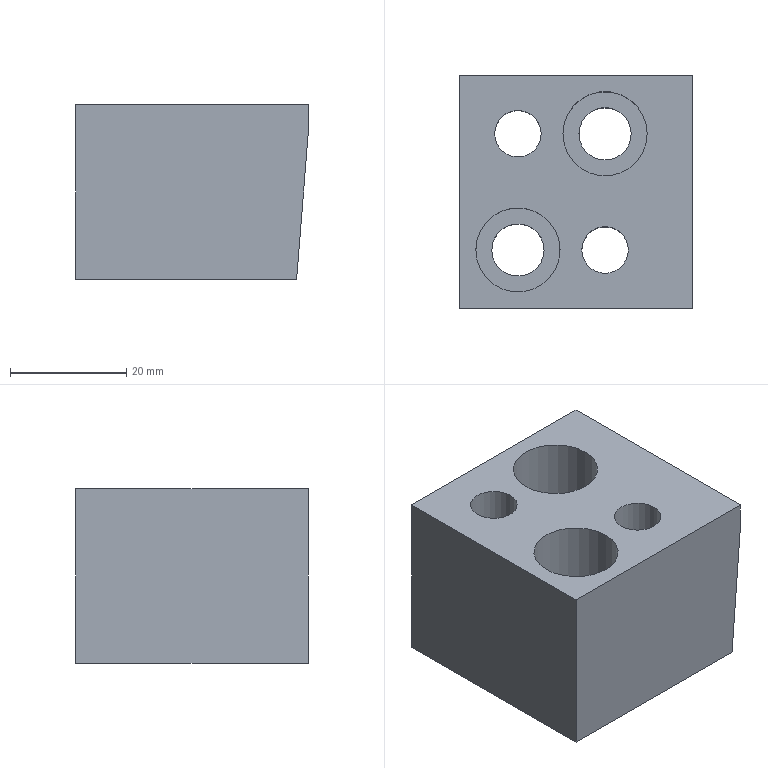Part | NX | features 23 2 | 1 solid | 15 faces | box 40 x 40 x 30 mm | volume 37933 mm3 | plane 9 | cylinder 6 | commonest cylinder face diameters 8.001 x2 9 x2 14.5 x2
STEP:
#1=CARTESIAN_POINT('',(3683.056,10.,-3.5));
#2=VERTEX_POINT('',#1);
#3=CARTESIAN_POINT('',(3675.806,10.,-3.5));
#4=DIRECTION('',(0.,0.,-1.));
#5=DIRECTION('',(1.,0.,0.));
#6=AXIS2_PLACEMENT_3D('',#3,#4,#5);
#7=CIRCLE('',#6,7.25);
#8=EDGE_CURVE('',#2,#2,#7,.T.);
#9=ORIENTED_EDGE('',*,*,#8,.T.);
#10=EDGE_LOOP('',(#9));
#11=FACE_BOUND('',#10,.T.);
#12=CARTESIAN_POINT('',(3690.806,-20.,-3.5));
#13=VERTEX_POINT('',#12);
#14=CARTESIAN_POINT('',(3650.806,-20.,-3.5));
#15=VERTEX_POINT('',#14);
#16=CARTESIAN_POINT('',(3675.806,-20.,-3.5));
#17=DIRECTION('',(-1.,0.,0.));
#18=VECTOR('',#17,1000.);
#19=LINE('',#16,#18);
#20=EDGE_CURVE('',#13,#15,#19,.T.);
#21=ORIENTED_EDGE('',*,*,#20,.F.);
#22=CARTESIAN_POINT('',(3690.806,20.,-3.5));
#23=VERTEX_POINT('',#22);
#24=CARTESIAN_POINT('',(3690.806,0.,-3.5));
#25=DIRECTION('',(0.,-1.,0.));
#26=VECTOR('',#25,1000.);
#27=LINE('',#24,#26);
#28=EDGE_CURVE('',#23,#13,#27,.T.);
#29=ORIENTED_EDGE('',*,*,#28,.F.);
#30=CARTESIAN_POINT('',(3650.806,20.,-3.5));
#31=VERTEX_POINT('',#30);
#32=CARTESIAN_POINT('',(3675.806,20.,-3.5));
#33=DIRECTION('',(1.,0.,0.));
#34=VECTOR('',#33,1000.);
#35=LINE('',#32,#34);
#36=EDGE_CURVE('',#31,#23,#35,.T.);
#37=ORIENTED_EDGE('',*,*,#36,.F.);
#38=CARTESIAN_POINT('',(3650.806,0.,-3.5));
#39=DIRECTION('',(0.,1.,0.));
#40=VECTOR('',#39,1000.);
#41=LINE('',#38,#40);
#42=EDGE_CURVE('',#15,#31,#41,.T.);
#43=ORIENTED_EDGE('',*,*,#42,.F.);
#44=EDGE_LOOP('',(#21,#29,#37,#43));
#45=FACE_BOUND('',#44,.T.);
#46=CARTESIAN_POINT('',(3664.807,10.,-3.5));
#47=VERTEX_POINT('',#46);
#48=CARTESIAN_POINT('',(3660.806,10.,-3.5));
#49=DIRECTION('',(0.,0.,1.));
#50=DIRECTION('',(1.,0.,0.));
#51=AXIS2_PLACEMENT_3D('',#48,#49,#50);
#52=CIRCLE('',#51,4.);
#53=EDGE_CURVE('',#47,#47,#52,.T.);
#54=ORIENTED_EDGE('',*,*,#53,.F.);
#55=EDGE_LOOP('',(#54));
#56=FACE_BOUND('',#55,.T.);
#57=CARTESIAN_POINT('',(3679.807,-10.,-3.5));
#58=VERTEX_POINT('',#57);
#59=CARTESIAN_POINT('',(3675.806,-10.,-3.5));
#60=DIRECTION('',(0.,0.,1.));
#61=DIRECTION('',(1.,0.,0.));
#62=AXIS2_PLACEMENT_3D('',#59,#60,#61);
#63=CIRCLE('',#62,4.);
#64=EDGE_CURVE('',#58,#58,#63,.T.);
#65=ORIENTED_EDGE('',*,*,#64,.F.);
#66=EDGE_LOOP('',(#65));
#67=FACE_BOUND('',#66,.T.);
#68=CARTESIAN_POINT('',(3668.056,-10.,-3.5));
#69=VERTEX_POINT('',#68);
#70=CARTESIAN_POINT('',(3660.806,-10.,-3.5));
#71=DIRECTION('',(0.,0.,-1.));
#72=DIRECTION('',(1.,0.,0.));
#73=AXIS2_PLACEMENT_3D('',#70,#71,#72);
#74=CIRCLE('',#73,7.25);
#75=EDGE_CURVE('',#69,#69,#74,.T.);
#76=ORIENTED_EDGE('',*,*,#75,.T.);
#77=EDGE_LOOP('',(#76));
#78=FACE_BOUND('',#77,.T.);
#79=CARTESIAN_POINT('',(3675.806,0.,-3.5));
#80=DIRECTION('',(0.,0.,1.));
#81=DIRECTION('',(-1.,0.,0.));
#82=AXIS2_PLACEMENT_3D('',#79,#80,#81);
#83=PLANE('',#82);
#84=ADVANCED_FACE('',(#11,#45,#56,#67,#78),#83,.T.);
#85=CARTESIAN_POINT('',(3650.806,-20.,-33.5));
#86=VERTEX_POINT('',#85);
#87=CARTESIAN_POINT('',(3688.806,-20.,-33.5));
#88=VERTEX_POINT('',#87);
#89=CARTESIAN_POINT('',(3675.806,-20.,-33.5));
#90=DIRECTION('',(1.,0.,0.));
#91=VECTOR('',#90,1000.);
#92=LINE('',#89,#91);
#93=EDGE_CURVE('',#86,#88,#92,.T.);
#94=ORIENTED_EDGE('',*,*,#93,.T.);
#95=CARTESIAN_POINT('',(3690.806,-20.,-8.5));
#96=VERTEX_POINT('',#95);
#97=CARTESIAN_POINT('',(3688.724,-20.,-34.533));
#98=DIRECTION('',(0.07975,0.,0.9968));
#99=VECTOR('',#98,1000.);
#100=LINE('',#97,#99);
#101=EDGE_CURVE('',#88,#96,#100,.T.);
#102=ORIENTED_EDGE('',*,*,#101,.T.);
#103=CARTESIAN_POINT('',(3690.806,-20.,-33.5));
#104=DIRECTION('',(0.,0.,1.));
#105=VECTOR('',#104,1000.);
#106=LINE('',#103,#105);
#107=EDGE_CURVE('',#96,#13,#106,.T.);
#108=ORIENTED_EDGE('',*,*,#107,.T.);
#109=ORIENTED_EDGE('',*,*,#20,.T.);
#110=CARTESIAN_POINT('',(3650.806,-20.,-33.5));
#111=DIRECTION('',(0.,0.,1.));
#112=VECTOR('',#111,1000.);
#113=LINE('',#110,#112);
#114=EDGE_CURVE('',#86,#15,#113,.T.);
#115=ORIENTED_EDGE('',*,*,#114,.F.);
#116=EDGE_LOOP('',(#94,#102,#108,#109,#115));
#117=FACE_BOUND('',#116,.T.);
#118=CARTESIAN_POINT('',(3675.806,-20.,-33.5));
#119=DIRECTION('',(0.,-1.,0.));
#120=DIRECTION('',(0.,0.,1.));
#121=AXIS2_PLACEMENT_3D('',#118,#119,#120);
#122=PLANE('',#121);
#123=ADVANCED_FACE('',(#117),#122,.T.);
#124=ORIENTED_EDGE('',*,*,#114,.T.);
#125=ORIENTED_EDGE('',*,*,#42,.T.);
#126=CARTESIAN_POINT('',(3650.806,20.,-33.5));
#127=VERTEX_POINT('',#126);
#128=CARTESIAN_POINT('',(3650.806,20.,-33.5));
#129=DIRECTION('',(0.,0.,1.));
#130=VECTOR('',#129,1000.);
#131=LINE('',#128,#130);
#132=EDGE_CURVE('',#127,#31,#131,.T.);
#133=ORIENTED_EDGE('',*,*,#132,.F.);
#134=CARTESIAN_POINT('',(3650.806,0.,-33.5));
#135=DIRECTION('',(0.,-1.,0.));
#136=VECTOR('',#135,1000.);
#137=LINE('',#134,#136);
#138=EDGE_CURVE('',#127,#86,#137,.T.);
#139=ORIENTED_EDGE('',*,*,#138,.T.);
#140=EDGE_LOOP('',(#124,#125,#133,#139));
#141=FACE_BOUND('',#140,.T.);
#142=CARTESIAN_POINT('',(3650.806,0.,-33.5));
#143=DIRECTION('',(-1.,0.,0.));
#144=DIRECTION('',(0.,0.,-1.));
#145=AXIS2_PLACEMENT_3D('',#142,#143,#144);
#146=PLANE('',#145);
#147=ADVANCED_FACE('',(#141),#146,.T.);
#148=CARTESIAN_POINT('',(3690.806,20.,-8.5));
#149=VERTEX_POINT('',#148);
#150=CARTESIAN_POINT('',(3690.806,20.,-33.5));
#151=DIRECTION('',(0.,0.,1.));
#152=VECTOR('',#151,1000.);
#153=LINE('',#150,#152);
#154=EDGE_CURVE('',#149,#23,#153,.T.);
#155=ORIENTED_EDGE('',*,*,#154,.F.);
#156=CARTESIAN_POINT('',(3688.806,20.,-33.5));
#157=VERTEX_POINT('',#156);
#158=CARTESIAN_POINT('',(3688.724,20.,-34.533));
#159=DIRECTION('',(-0.07975,0.,-0.9968));
#160=VECTOR('',#159,1000.);
#161=LINE('',#158,#160);
#162=EDGE_CURVE('',#149,#157,#161,.T.);
#163=ORIENTED_EDGE('',*,*,#162,.T.);
#164=CARTESIAN_POINT('',(3675.806,20.,-33.5));
#165=DIRECTION('',(-1.,0.,0.));
#166=VECTOR('',#165,1000.);
#167=LINE('',#164,#166);
#168=EDGE_CURVE('',#157,#127,#167,.T.);
#169=ORIENTED_EDGE('',*,*,#168,.T.);
#170=ORIENTED_EDGE('',*,*,#132,.T.);
#171=ORIENTED_EDGE('',*,*,#36,.T.);
#172=EDGE_LOOP('',(#155,#163,#169,#170,#171));
#173=FACE_BOUND('',#172,.T.);
#174=CARTESIAN_POINT('',(3675.806,20.,-33.5));
#175=DIRECTION('',(0.,1.,0.));
#176=DIRECTION('',(0.,0.,-1.));
#177=AXIS2_PLACEMENT_3D('',#174,#175,#176);
#178=PLANE('',#177);
#179=ADVANCED_FACE('',(#173),#178,.T.);
#180=CARTESIAN_POINT('',(3656.306,-10.,-33.5));
#181=VERTEX_POINT('',#180);
#182=CARTESIAN_POINT('',(3660.806,-10.,-33.5));
#183=DIRECTION('',(0.,0.,-1.));
#184=DIRECTION('',(-1.,0.,0.));
#185=AXIS2_PLACEMENT_3D('',#182,#183,#184);
#186=CIRCLE('',#185,4.5);
#187=EDGE_CURVE('',#181,#181,#186,.T.);
#188=ORIENTED_EDGE('',*,*,#187,.F.);
#189=EDGE_LOOP('',(#188));
#190=FACE_BOUND('',#189,.T.);
#191=CARTESIAN_POINT('',(3671.806,-10.,-33.5));
#192=VERTEX_POINT('',#191);
#193=CARTESIAN_POINT('',(3675.806,-10.,-33.5));
#194=DIRECTION('',(0.,0.,-1.));
#195=DIRECTION('',(-1.,0.,0.));
#196=AXIS2_PLACEMENT_3D('',#193,#194,#195);
#197=CIRCLE('',#196,4.);
#198=EDGE_CURVE('',#192,#192,#197,.T.);
#199=ORIENTED_EDGE('',*,*,#198,.F.);
#200=EDGE_LOOP('',(#199));
#201=FACE_BOUND('',#200,.T.);
#202=CARTESIAN_POINT('',(3656.806,10.,-33.5));
#203=VERTEX_POINT('',#202);
#204=CARTESIAN_POINT('',(3660.806,10.,-33.5));
#205=DIRECTION('',(0.,0.,-1.));
#206=DIRECTION('',(-1.,0.,0.));
#207=AXIS2_PLACEMENT_3D('',#204,#205,#206);
#208=CIRCLE('',#207,4.);
#209=EDGE_CURVE('',#203,#203,#208,.T.);
#210=ORIENTED_EDGE('',*,*,#209,.F.);
#211=EDGE_LOOP('',(#210));
#212=FACE_BOUND('',#211,.T.);
#213=CARTESIAN_POINT('',(3671.306,10.,-33.5));
#214=VERTEX_POINT('',#213);
#215=CARTESIAN_POINT('',(3675.806,10.,-33.5));
#216=DIRECTION('',(0.,0.,-1.));
#217=DIRECTION('',(-1.,0.,0.));
#218=AXIS2_PLACEMENT_3D('',#215,#216,#217);
#219=CIRCLE('',#218,4.5);
#220=EDGE_CURVE('',#214,#214,#219,.T.);
#221=ORIENTED_EDGE('',*,*,#220,.F.);
#222=EDGE_LOOP('',(#221));
#223=FACE_BOUND('',#222,.T.);
#224=ORIENTED_EDGE('',*,*,#168,.F.);
#225=CARTESIAN_POINT('',(3688.806,0.,-33.5));
#226=DIRECTION('',(0.,-1.,0.));
#227=VECTOR('',#226,1000.);
#228=LINE('',#225,#227);
#229=EDGE_CURVE('',#157,#88,#228,.T.);
#230=ORIENTED_EDGE('',*,*,#229,.T.);
#231=ORIENTED_EDGE('',*,*,#93,.F.);
#232=ORIENTED_EDGE('',*,*,#138,.F.);
#233=EDGE_LOOP('',(#224,#230,#231,#232));
#234=FACE_BOUND('',#233,.T.);
#235=CARTESIAN_POINT('',(3675.806,0.,-33.5));
#236=DIRECTION('',(0.,0.,-1.));
#237=DIRECTION('',(1.,0.,0.));
#238=AXIS2_PLACEMENT_3D('',#235,#236,#237);
#239=PLANE('',#238);
#240=ADVANCED_FACE('',(#190,#201,#212,#223,#234),#239,.T.);
#241=ORIENTED_EDGE('',*,*,#107,.F.);
#242=CARTESIAN_POINT('',(3690.806,0.,-8.5));
#243=DIRECTION('',(0.,1.,0.));
#244=VECTOR('',#243,1000.);
#245=LINE('',#242,#244);
#246=EDGE_CURVE('',#96,#149,#245,.T.);
#247=ORIENTED_EDGE('',*,*,#246,.T.);
#248=ORIENTED_EDGE('',*,*,#154,.T.);
#249=ORIENTED_EDGE('',*,*,#28,.T.);
#250=EDGE_LOOP('',(#241,#247,#248,#249));
#251=FACE_BOUND('',#250,.T.);
#252=CARTESIAN_POINT('',(3690.806,0.,-33.5));
#253=DIRECTION('',(1.,0.,0.));
#254=DIRECTION('',(0.,0.,1.));
#255=AXIS2_PLACEMENT_3D('',#252,#253,#254);
#256=PLANE('',#255);
#257=ADVANCED_FACE('',(#251),#256,.T.);
#258=ORIENTED_EDGE('',*,*,#220,.T.);
#259=EDGE_LOOP('',(#258));
#260=FACE_BOUND('',#259,.T.);
#261=CARTESIAN_POINT('',(3671.306,10.,-14.5));
#262=VERTEX_POINT('',#261);
#263=CARTESIAN_POINT('',(3675.806,10.,-14.5));
#264=DIRECTION('',(0.,0.,-1.));
#265=DIRECTION('',(-1.,0.,0.));
#266=AXIS2_PLACEMENT_3D('',#263,#264,#265);
#267=CIRCLE('',#266,4.5);
#268=EDGE_CURVE('',#262,#262,#267,.T.);
#269=ORIENTED_EDGE('',*,*,#268,.F.);
#270=EDGE_LOOP('',(#269));
#271=FACE_BOUND('',#270,.T.);
#272=CARTESIAN_POINT('',(3675.806,10.,-1.5));
#273=DIRECTION('',(0.,0.,-1.));
#274=DIRECTION('',(-1.,0.,0.));
#275=AXIS2_PLACEMENT_3D('',#272,#273,#274);
#276=CYLINDRICAL_SURFACE('',#275,4.5);
#277=ADVANCED_FACE('',(#260,#271),#276,.F.);
#278=ORIENTED_EDGE('',*,*,#268,.T.);
#279=EDGE_LOOP('',(#278));
#280=FACE_BOUND('',#279,.T.);
#281=CARTESIAN_POINT('',(3683.056,10.,-14.5));
#282=VERTEX_POINT('',#281);
#283=CARTESIAN_POINT('',(3675.806,10.,-14.5));
#284=DIRECTION('',(0.,0.,-1.));
#285=DIRECTION('',(1.,0.,0.));
#286=AXIS2_PLACEMENT_3D('',#283,#284,#285);
#287=CIRCLE('',#286,7.25);
#288=EDGE_CURVE('',#282,#282,#287,.T.);
#289=ORIENTED_EDGE('',*,*,#288,.F.);
#290=EDGE_LOOP('',(#289));
#291=FACE_BOUND('',#290,.T.);
#292=CARTESIAN_POINT('',(3675.806,10.,-14.5));
#293=DIRECTION('',(0.,0.,-1.));
#294=DIRECTION('',(1.,0.,0.));
#295=AXIS2_PLACEMENT_3D('',#292,#293,#294);
#296=PLANE('',#295);
#297=ADVANCED_FACE('',(#280,#291),#296,.F.);
#298=ORIENTED_EDGE('',*,*,#288,.T.);
#299=EDGE_LOOP('',(#298));
#300=FACE_BOUND('',#299,.T.);
#301=ORIENTED_EDGE('',*,*,#8,.F.);
#302=EDGE_LOOP('',(#301));
#303=FACE_BOUND('',#302,.T.);
#304=CARTESIAN_POINT('',(3675.806,10.,-3.5));
#305=DIRECTION('',(0.,0.,-1.));
#306=DIRECTION('',(-1.,0.,0.));
#307=AXIS2_PLACEMENT_3D('',#304,#305,#306);
#308=CYLINDRICAL_SURFACE('',#307,7.25);
#309=ADVANCED_FACE('',(#300,#303),#308,.F.);
#310=ORIENTED_EDGE('',*,*,#53,.T.);
#311=EDGE_LOOP('',(#310));
#312=FACE_BOUND('',#311,.T.);
#313=ORIENTED_EDGE('',*,*,#209,.T.);
#314=EDGE_LOOP('',(#313));
#315=FACE_BOUND('',#314,.T.);
#316=CARTESIAN_POINT('',(3660.806,10.,-1.5));
#317=DIRECTION('',(0.,0.,-1.));
#318=DIRECTION('',(-1.,0.,0.));
#319=AXIS2_PLACEMENT_3D('',#316,#317,#318);
#320=CYLINDRICAL_SURFACE('',#319,4.);
#321=ADVANCED_FACE('',(#312,#315),#320,.F.);
#322=ORIENTED_EDGE('',*,*,#64,.T.);
#323=EDGE_LOOP('',(#322));
#324=FACE_BOUND('',#323,.T.);
#325=ORIENTED_EDGE('',*,*,#198,.T.);
#326=EDGE_LOOP('',(#325));
#327=FACE_BOUND('',#326,.T.);
#328=CARTESIAN_POINT('',(3675.806,-10.,-1.5));
#329=DIRECTION('',(0.,0.,-1.));
#330=DIRECTION('',(-1.,0.,0.));
#331=AXIS2_PLACEMENT_3D('',#328,#329,#330);
#332=CYLINDRICAL_SURFACE('',#331,4.);
#333=ADVANCED_FACE('',(#324,#327),#332,.F.);
#334=ORIENTED_EDGE('',*,*,#187,.T.);
#335=EDGE_LOOP('',(#334));
#336=FACE_BOUND('',#335,.T.);
#337=CARTESIAN_POINT('',(3656.306,-10.,-14.5));
#338=VERTEX_POINT('',#337);
#339=CARTESIAN_POINT('',(3660.806,-10.,-14.5));
#340=DIRECTION('',(0.,0.,-1.));
#341=DIRECTION('',(-1.,0.,0.));
#342=AXIS2_PLACEMENT_3D('',#339,#340,#341);
#343=CIRCLE('',#342,4.5);
#344=EDGE_CURVE('',#338,#338,#343,.T.);
#345=ORIENTED_EDGE('',*,*,#344,.F.);
#346=EDGE_LOOP('',(#345));
#347=FACE_BOUND('',#346,.T.);
#348=CARTESIAN_POINT('',(3660.806,-10.,-1.5));
#349=DIRECTION('',(0.,0.,-1.));
#350=DIRECTION('',(-1.,0.,0.));
#351=AXIS2_PLACEMENT_3D('',#348,#349,#350);
#352=CYLINDRICAL_SURFACE('',#351,4.5);
#353=ADVANCED_FACE('',(#336,#347),#352,.F.);
#354=ORIENTED_EDGE('',*,*,#344,.T.);
#355=EDGE_LOOP('',(#354));
#356=FACE_BOUND('',#355,.T.);
#357=CARTESIAN_POINT('',(3668.056,-10.,-14.5));
#358=VERTEX_POINT('',#357);
#359=CARTESIAN_POINT('',(3660.806,-10.,-14.5));
#360=DIRECTION('',(0.,0.,-1.));
#361=DIRECTION('',(1.,0.,0.));
#362=AXIS2_PLACEMENT_3D('',#359,#360,#361);
#363=CIRCLE('',#362,7.25);
#364=EDGE_CURVE('',#358,#358,#363,.T.);
#365=ORIENTED_EDGE('',*,*,#364,.F.);
#366=EDGE_LOOP('',(#365));
#367=FACE_BOUND('',#366,.T.);
#368=CARTESIAN_POINT('',(3660.806,-10.,-14.5));
#369=DIRECTION('',(0.,0.,-1.));
#370=DIRECTION('',(1.,0.,0.));
#371=AXIS2_PLACEMENT_3D('',#368,#369,#370);
#372=PLANE('',#371);
#373=ADVANCED_FACE('',(#356,#367),#372,.F.);
#374=ORIENTED_EDGE('',*,*,#364,.T.);
#375=EDGE_LOOP('',(#374));
#376=FACE_BOUND('',#375,.T.);
#377=ORIENTED_EDGE('',*,*,#75,.F.);
#378=EDGE_LOOP('',(#377));
#379=FACE_BOUND('',#378,.T.);
#380=CARTESIAN_POINT('',(3660.806,-10.,-3.5));
#381=DIRECTION('',(0.,0.,-1.));
#382=DIRECTION('',(-1.,0.,0.));
#383=AXIS2_PLACEMENT_3D('',#380,#381,#382);
#384=CYLINDRICAL_SURFACE('',#383,7.25);
#385=ADVANCED_FACE('',(#376,#379),#384,.F.);
#386=ORIENTED_EDGE('',*,*,#101,.F.);
#387=ORIENTED_EDGE('',*,*,#229,.F.);
#388=ORIENTED_EDGE('',*,*,#162,.F.);
#389=ORIENTED_EDGE('',*,*,#246,.F.);
#390=EDGE_LOOP('',(#386,#387,#388,#389));
#391=FACE_BOUND('',#390,.T.);
#392=CARTESIAN_POINT('',(3690.806,0.,-8.5));
#393=DIRECTION('',(-0.9968,0.,0.07975));
#394=DIRECTION('',(0.,-1.,0.));
#395=AXIS2_PLACEMENT_3D('',#392,#393,#394);
#396=PLANE('',#395);
#397=ADVANCED_FACE('',(#391),#396,.F.);
#398=CLOSED_SHELL('',(#84,#123,#147,#179,#240,#257,#277,#297,#309,#321,#333,#353,#373,#385,#397));
#399=MANIFOLD_SOLID_BREP('',#398);
#400=(LENGTH_UNIT()NAMED_UNIT(*)SI_UNIT(.MILLI.,.METRE.));
#401=UNCERTAINTY_MEASURE_WITH_UNIT(LENGTH_MEASURE(0.00001),#400,'','');
#402=(NAMED_UNIT(*)PLANE_ANGLE_UNIT()SI_UNIT($,.RADIAN.));
#403=(NAMED_UNIT(*)SI_UNIT($,.STERADIAN.)SOLID_ANGLE_UNIT());
#404=(GEOMETRIC_REPRESENTATION_CONTEXT(3)GLOBAL_UNCERTAINTY_ASSIGNED_CONTEXT((#401))GLOBAL_UNIT_ASSIGNED_CONTEXT((#400,#402,#403))REPRESENTATION_CONTEXT('',''));
#405=ADVANCED_BREP_SHAPE_REPRESENTATION('',(#399),#404);